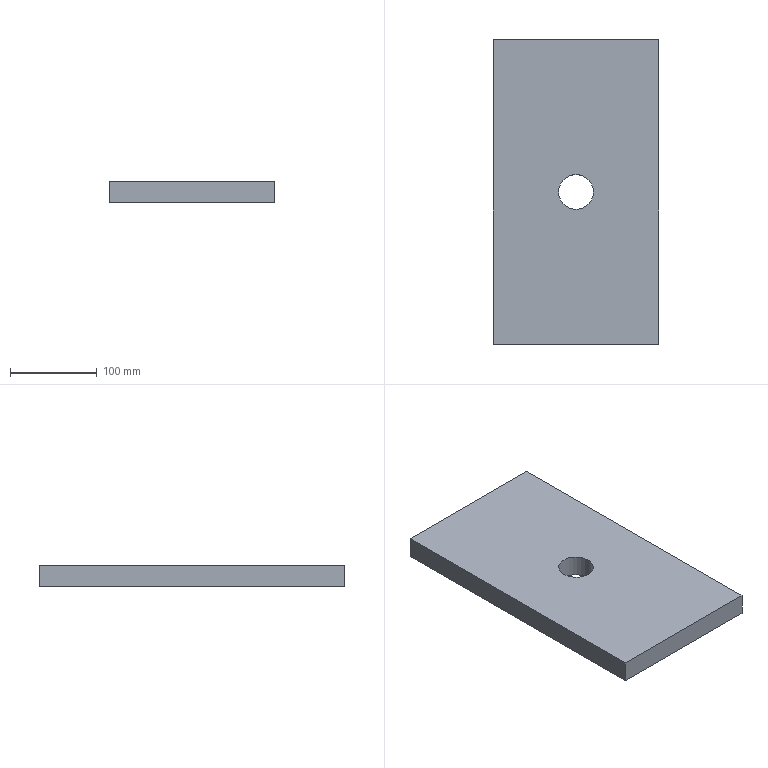Part | STEP file | Sprocket mounting plate XG | 1 solid | 8 faces | box 190 x 350 x 25 mm | volume 1631084 mm3 | plane 6 | cylinder 2 | commonest cylinder face diameters 40 x2
STEP:
#1=CARTESIAN_POINT('',(0.,0.,0.));
#2=DIRECTION('',(0.,0.,1.));
#3=DIRECTION('',(1.,0.,0.));
#4=AXIS2_PLACEMENT_3D('',#1,#2,#3);
#5=CARTESIAN_POINT('',(20.,0.,0.));
#6=VERTEX_POINT('',#5);
#7=CARTESIAN_POINT('',(20.,0.,25.));
#8=VERTEX_POINT('',#7);
#9=CARTESIAN_POINT('',(20.,0.,0.));
#10=DIRECTION('',(0.,0.,1.));
#11=VECTOR('',#10,1.);
#12=LINE('',#9,#11);
#13=CARTESIAN_POINT('',(0.,0.,0.));
#14=DIRECTION('',(0.,0.,1.));
#15=DIRECTION('',(1.,0.,0.));
#16=AXIS2_PLACEMENT_3D('',#13,#14,#15);
#17=CYLINDRICAL_SURFACE('',#16,20.);
#18=CARTESIAN_POINT('',(6.283,0.));
#19=DIRECTION('',(0.,1.));
#20=VECTOR('',#19,1.);
#21=LINE('',#18,#20);
#22=(GEOMETRIC_REPRESENTATION_CONTEXT(2)PARAMETRIC_REPRESENTATION_CONTEXT()REPRESENTATION_CONTEXT('',''));
#23=DEFINITIONAL_REPRESENTATION('',(#21),#22);
#24=PCURVE('',#17,#23);
#25=CARTESIAN_POINT('',(0.,0.,0.));
#26=DIRECTION('',(0.,0.,1.));
#27=DIRECTION('',(1.,0.,0.));
#28=AXIS2_PLACEMENT_3D('',#25,#26,#27);
#29=CYLINDRICAL_SURFACE('',#28,20.);
#30=CARTESIAN_POINT('',(0.,0.));
#31=DIRECTION('',(0.,1.));
#32=VECTOR('',#31,1.);
#33=LINE('',#30,#32);
#34=(GEOMETRIC_REPRESENTATION_CONTEXT(2)PARAMETRIC_REPRESENTATION_CONTEXT()REPRESENTATION_CONTEXT('',''));
#35=DEFINITIONAL_REPRESENTATION('',(#33),#34);
#36=PCURVE('',#29,#35);
#37=SURFACE_CURVE('',#12,(#24,#36),.PCURVE_S1.);
#38=EDGE_CURVE('',#6,#8,#37,.T.);
#39=ORIENTED_EDGE('',*,*,#38,.T.);
#40=CARTESIAN_POINT('',(-20.,0.,25.));
#41=VERTEX_POINT('',#40);
#42=CARTESIAN_POINT('',(0.,0.,25.));
#43=DIRECTION('',(0.,0.,1.));
#44=DIRECTION('',(1.,0.,0.));
#45=AXIS2_PLACEMENT_3D('',#42,#43,#44);
#46=CIRCLE('',#45,20.);
#47=CARTESIAN_POINT('',(0.,25.));
#48=DIRECTION('',(1.,0.));
#49=VECTOR('',#48,1.);
#50=LINE('',#47,#49);
#51=(GEOMETRIC_REPRESENTATION_CONTEXT(2)PARAMETRIC_REPRESENTATION_CONTEXT()REPRESENTATION_CONTEXT('',''));
#52=DEFINITIONAL_REPRESENTATION('',(#50),#51);
#53=PCURVE('',#17,#52);
#54=CARTESIAN_POINT('',(0.,0.,25.));
#55=DIRECTION('',(0.,0.,1.));
#56=DIRECTION('',(1.,0.,0.));
#57=AXIS2_PLACEMENT_3D('',#54,#55,#56);
#58=PLANE('',#57);
#59=CARTESIAN_POINT('',(0.,0.));
#60=DIRECTION('',(1.,0.));
#61=AXIS2_PLACEMENT_2D('',#59,#60);
#62=CIRCLE('',#61,20.);
#63=(GEOMETRIC_REPRESENTATION_CONTEXT(2)PARAMETRIC_REPRESENTATION_CONTEXT()REPRESENTATION_CONTEXT('',''));
#64=DEFINITIONAL_REPRESENTATION('',(#62),#63);
#65=PCURVE('',#58,#64);
#66=SURFACE_CURVE('',#46,(#53,#65),.PCURVE_S1.);
#67=EDGE_CURVE('',#41,#8,#66,.T.);
#68=ORIENTED_EDGE('',*,*,#67,.F.);
#69=CARTESIAN_POINT('',(-20.,0.,0.));
#70=VERTEX_POINT('',#69);
#71=CARTESIAN_POINT('',(-20.,0.,0.));
#72=DIRECTION('',(0.,0.,1.));
#73=VECTOR('',#72,1.);
#74=LINE('',#71,#73);
#75=CARTESIAN_POINT('',(3.142,0.));
#76=DIRECTION('',(0.,1.));
#77=VECTOR('',#76,1.);
#78=LINE('',#75,#77);
#79=(GEOMETRIC_REPRESENTATION_CONTEXT(2)PARAMETRIC_REPRESENTATION_CONTEXT()REPRESENTATION_CONTEXT('',''));
#80=DEFINITIONAL_REPRESENTATION('',(#78),#79);
#81=PCURVE('',#17,#80);
#82=CARTESIAN_POINT('',(3.142,0.));
#83=DIRECTION('',(0.,1.));
#84=VECTOR('',#83,1.);
#85=LINE('',#82,#84);
#86=(GEOMETRIC_REPRESENTATION_CONTEXT(2)PARAMETRIC_REPRESENTATION_CONTEXT()REPRESENTATION_CONTEXT('',''));
#87=DEFINITIONAL_REPRESENTATION('',(#85),#86);
#88=PCURVE('',#29,#87);
#89=SURFACE_CURVE('',#74,(#81,#88),.PCURVE_S1.);
#90=EDGE_CURVE('',#70,#41,#89,.T.);
#91=ORIENTED_EDGE('',*,*,#90,.F.);
#92=CARTESIAN_POINT('',(0.,0.,0.));
#93=DIRECTION('',(0.,0.,1.));
#94=DIRECTION('',(1.,0.,0.));
#95=AXIS2_PLACEMENT_3D('',#92,#93,#94);
#96=CIRCLE('',#95,20.);
#97=CARTESIAN_POINT('',(0.,0.));
#98=DIRECTION('',(1.,0.));
#99=VECTOR('',#98,1.);
#100=LINE('',#97,#99);
#101=(GEOMETRIC_REPRESENTATION_CONTEXT(2)PARAMETRIC_REPRESENTATION_CONTEXT()REPRESENTATION_CONTEXT('',''));
#102=DEFINITIONAL_REPRESENTATION('',(#100),#101);
#103=PCURVE('',#17,#102);
#104=CARTESIAN_POINT('',(0.,0.,0.));
#105=DIRECTION('',(0.,0.,1.));
#106=DIRECTION('',(1.,0.,0.));
#107=AXIS2_PLACEMENT_3D('',#104,#105,#106);
#108=PLANE('',#107);
#109=CARTESIAN_POINT('',(0.,0.));
#110=DIRECTION('',(1.,0.));
#111=AXIS2_PLACEMENT_2D('',#109,#110);
#112=CIRCLE('',#111,20.);
#113=(GEOMETRIC_REPRESENTATION_CONTEXT(2)PARAMETRIC_REPRESENTATION_CONTEXT()REPRESENTATION_CONTEXT('',''));
#114=DEFINITIONAL_REPRESENTATION('',(#112),#113);
#115=PCURVE('',#108,#114);
#116=SURFACE_CURVE('',#96,(#103,#115),.PCURVE_S1.);
#117=EDGE_CURVE('',#70,#6,#116,.T.);
#118=ORIENTED_EDGE('',*,*,#117,.T.);
#119=EDGE_LOOP('',(#39,#68,#91,#118));
#120=FACE_BOUND('',#119,.F.);
#121=ADVANCED_FACE('',(#120),#17,.F.);
#122=CARTESIAN_POINT('',(-95.,175.,0.));
#123=VERTEX_POINT('',#122);
#124=CARTESIAN_POINT('',(-95.,-175.,0.));
#125=VERTEX_POINT('',#124);
#126=CARTESIAN_POINT('',(-95.,175.,0.));
#127=DIRECTION('',(0.,-1.,0.));
#128=VECTOR('',#127,1.);
#129=LINE('',#126,#128);
#130=CARTESIAN_POINT('',(-95.,175.,25.));
#131=DIRECTION('',(1.,0.,0.));
#132=DIRECTION('',(0.,0.,-1.));
#133=AXIS2_PLACEMENT_3D('',#130,#131,#132);
#134=PLANE('',#133);
#135=CARTESIAN_POINT('',(25.,0.));
#136=DIRECTION('',(0.,-1.));
#137=VECTOR('',#136,1.);
#138=LINE('',#135,#137);
#139=(GEOMETRIC_REPRESENTATION_CONTEXT(2)PARAMETRIC_REPRESENTATION_CONTEXT()REPRESENTATION_CONTEXT('',''));
#140=DEFINITIONAL_REPRESENTATION('',(#138),#139);
#141=PCURVE('',#134,#140);
#142=CARTESIAN_POINT('',(-95.,175.));
#143=DIRECTION('',(0.,-1.));
#144=VECTOR('',#143,1.);
#145=LINE('',#142,#144);
#146=(GEOMETRIC_REPRESENTATION_CONTEXT(2)PARAMETRIC_REPRESENTATION_CONTEXT()REPRESENTATION_CONTEXT('',''));
#147=DEFINITIONAL_REPRESENTATION('',(#145),#146);
#148=PCURVE('',#108,#147);
#149=SURFACE_CURVE('',#129,(#141,#148),.PCURVE_S1.);
#150=EDGE_CURVE('',#123,#125,#149,.T.);
#151=ORIENTED_EDGE('',*,*,#150,.T.);
#152=CARTESIAN_POINT('',(-95.,-175.,25.));
#153=VERTEX_POINT('',#152);
#154=CARTESIAN_POINT('',(-95.,-175.,25.));
#155=DIRECTION('',(0.,0.,-1.));
#156=VECTOR('',#155,1.);
#157=LINE('',#154,#156);
#158=CARTESIAN_POINT('',(0.,-350.));
#159=DIRECTION('',(1.,0.));
#160=VECTOR('',#159,1.);
#161=LINE('',#158,#160);
#162=(GEOMETRIC_REPRESENTATION_CONTEXT(2)PARAMETRIC_REPRESENTATION_CONTEXT()REPRESENTATION_CONTEXT('',''));
#163=DEFINITIONAL_REPRESENTATION('',(#161),#162);
#164=PCURVE('',#134,#163);
#165=CARTESIAN_POINT('',(-95.,-175.,25.));
#166=DIRECTION('',(0.,1.,0.));
#167=DIRECTION('',(0.,0.,1.));
#168=AXIS2_PLACEMENT_3D('',#165,#166,#167);
#169=PLANE('',#168);
#170=CARTESIAN_POINT('',(0.,0.));
#171=DIRECTION('',(-1.,0.));
#172=VECTOR('',#171,1.);
#173=LINE('',#170,#172);
#174=(GEOMETRIC_REPRESENTATION_CONTEXT(2)PARAMETRIC_REPRESENTATION_CONTEXT()REPRESENTATION_CONTEXT('',''));
#175=DEFINITIONAL_REPRESENTATION('',(#173),#174);
#176=PCURVE('',#169,#175);
#177=SURFACE_CURVE('',#157,(#164,#176),.PCURVE_S1.);
#178=EDGE_CURVE('',#153,#125,#177,.T.);
#179=ORIENTED_EDGE('',*,*,#178,.F.);
#180=CARTESIAN_POINT('',(-95.,175.,25.));
#181=VERTEX_POINT('',#180);
#182=CARTESIAN_POINT('',(-95.,175.,25.));
#183=DIRECTION('',(0.,-1.,0.));
#184=VECTOR('',#183,1.);
#185=LINE('',#182,#184);
#186=CARTESIAN_POINT('',(0.,0.));
#187=DIRECTION('',(0.,-1.));
#188=VECTOR('',#187,1.);
#189=LINE('',#186,#188);
#190=(GEOMETRIC_REPRESENTATION_CONTEXT(2)PARAMETRIC_REPRESENTATION_CONTEXT()REPRESENTATION_CONTEXT('',''));
#191=DEFINITIONAL_REPRESENTATION('',(#189),#190);
#192=PCURVE('',#134,#191);
#193=CARTESIAN_POINT('',(-95.,175.));
#194=DIRECTION('',(0.,-1.));
#195=VECTOR('',#194,1.);
#196=LINE('',#193,#195);
#197=(GEOMETRIC_REPRESENTATION_CONTEXT(2)PARAMETRIC_REPRESENTATION_CONTEXT()REPRESENTATION_CONTEXT('',''));
#198=DEFINITIONAL_REPRESENTATION('',(#196),#197);
#199=PCURVE('',#58,#198);
#200=SURFACE_CURVE('',#185,(#192,#199),.PCURVE_S1.);
#201=EDGE_CURVE('',#181,#153,#200,.T.);
#202=ORIENTED_EDGE('',*,*,#201,.F.);
#203=CARTESIAN_POINT('',(-95.,175.,25.));
#204=DIRECTION('',(0.,0.,-1.));
#205=VECTOR('',#204,1.);
#206=LINE('',#203,#205);
#207=CARTESIAN_POINT('',(0.,0.));
#208=DIRECTION('',(1.,0.));
#209=VECTOR('',#208,1.);
#210=LINE('',#207,#209);
#211=(GEOMETRIC_REPRESENTATION_CONTEXT(2)PARAMETRIC_REPRESENTATION_CONTEXT()REPRESENTATION_CONTEXT('',''));
#212=DEFINITIONAL_REPRESENTATION('',(#210),#211);
#213=PCURVE('',#134,#212);
#214=CARTESIAN_POINT('',(-95.,175.,25.));
#215=DIRECTION('',(0.,-1.,0.));
#216=DIRECTION('',(0.,0.,-1.));
#217=AXIS2_PLACEMENT_3D('',#214,#215,#216);
#218=PLANE('',#217);
#219=CARTESIAN_POINT('',(0.,0.));
#220=DIRECTION('',(1.,0.));
#221=VECTOR('',#220,1.);
#222=LINE('',#219,#221);
#223=(GEOMETRIC_REPRESENTATION_CONTEXT(2)PARAMETRIC_REPRESENTATION_CONTEXT()REPRESENTATION_CONTEXT('',''));
#224=DEFINITIONAL_REPRESENTATION('',(#222),#223);
#225=PCURVE('',#218,#224);
#226=SURFACE_CURVE('',#206,(#213,#225),.PCURVE_S1.);
#227=EDGE_CURVE('',#181,#123,#226,.T.);
#228=ORIENTED_EDGE('',*,*,#227,.T.);
#229=EDGE_LOOP('',(#151,#179,#202,#228));
#230=FACE_BOUND('',#229,.T.);
#231=ADVANCED_FACE('',(#230),#134,.F.);
#232=CARTESIAN_POINT('',(95.,-175.,0.));
#233=VERTEX_POINT('',#232);
#234=CARTESIAN_POINT('',(-95.,-175.,0.));
#235=DIRECTION('',(1.,0.,0.));
#236=VECTOR('',#235,1.);
#237=LINE('',#234,#236);
#238=CARTESIAN_POINT('',(-25.,0.));
#239=DIRECTION('',(0.,1.));
#240=VECTOR('',#239,1.);
#241=LINE('',#238,#240);
#242=(GEOMETRIC_REPRESENTATION_CONTEXT(2)PARAMETRIC_REPRESENTATION_CONTEXT()REPRESENTATION_CONTEXT('',''));
#243=DEFINITIONAL_REPRESENTATION('',(#241),#242);
#244=PCURVE('',#169,#243);
#245=CARTESIAN_POINT('',(-95.,-175.));
#246=DIRECTION('',(1.,0.));
#247=VECTOR('',#246,1.);
#248=LINE('',#245,#247);
#249=(GEOMETRIC_REPRESENTATION_CONTEXT(2)PARAMETRIC_REPRESENTATION_CONTEXT()REPRESENTATION_CONTEXT('',''));
#250=DEFINITIONAL_REPRESENTATION('',(#248),#249);
#251=PCURVE('',#108,#250);
#252=SURFACE_CURVE('',#237,(#244,#251),.PCURVE_S1.);
#253=EDGE_CURVE('',#125,#233,#252,.T.);
#254=ORIENTED_EDGE('',*,*,#253,.T.);
#255=CARTESIAN_POINT('',(95.,-175.,25.));
#256=VERTEX_POINT('',#255);
#257=CARTESIAN_POINT('',(95.,-175.,25.));
#258=DIRECTION('',(0.,0.,-1.));
#259=VECTOR('',#258,1.);
#260=LINE('',#257,#259);
#261=CARTESIAN_POINT('',(0.,190.));
#262=DIRECTION('',(-1.,0.));
#263=VECTOR('',#262,1.);
#264=LINE('',#261,#263);
#265=(GEOMETRIC_REPRESENTATION_CONTEXT(2)PARAMETRIC_REPRESENTATION_CONTEXT()REPRESENTATION_CONTEXT('',''));
#266=DEFINITIONAL_REPRESENTATION('',(#264),#265);
#267=PCURVE('',#169,#266);
#268=CARTESIAN_POINT('',(95.,175.,25.));
#269=DIRECTION('',(-1.,0.,0.));
#270=DIRECTION('',(0.,0.,1.));
#271=AXIS2_PLACEMENT_3D('',#268,#269,#270);
#272=PLANE('',#271);
#273=CARTESIAN_POINT('',(0.,-350.));
#274=DIRECTION('',(-1.,0.));
#275=VECTOR('',#274,1.);
#276=LINE('',#273,#275);
#277=(GEOMETRIC_REPRESENTATION_CONTEXT(2)PARAMETRIC_REPRESENTATION_CONTEXT()REPRESENTATION_CONTEXT('',''));
#278=DEFINITIONAL_REPRESENTATION('',(#276),#277);
#279=PCURVE('',#272,#278);
#280=SURFACE_CURVE('',#260,(#267,#279),.PCURVE_S1.);
#281=EDGE_CURVE('',#256,#233,#280,.T.);
#282=ORIENTED_EDGE('',*,*,#281,.F.);
#283=CARTESIAN_POINT('',(-95.,-175.,25.));
#284=DIRECTION('',(1.,0.,0.));
#285=VECTOR('',#284,1.);
#286=LINE('',#283,#285);
#287=CARTESIAN_POINT('',(0.,0.));
#288=DIRECTION('',(0.,1.));
#289=VECTOR('',#288,1.);
#290=LINE('',#287,#289);
#291=(GEOMETRIC_REPRESENTATION_CONTEXT(2)PARAMETRIC_REPRESENTATION_CONTEXT()REPRESENTATION_CONTEXT('',''));
#292=DEFINITIONAL_REPRESENTATION('',(#290),#291);
#293=PCURVE('',#169,#292);
#294=CARTESIAN_POINT('',(-95.,-175.));
#295=DIRECTION('',(1.,0.));
#296=VECTOR('',#295,1.);
#297=LINE('',#294,#296);
#298=(GEOMETRIC_REPRESENTATION_CONTEXT(2)PARAMETRIC_REPRESENTATION_CONTEXT()REPRESENTATION_CONTEXT('',''));
#299=DEFINITIONAL_REPRESENTATION('',(#297),#298);
#300=PCURVE('',#58,#299);
#301=SURFACE_CURVE('',#286,(#293,#300),.PCURVE_S1.);
#302=EDGE_CURVE('',#153,#256,#301,.T.);
#303=ORIENTED_EDGE('',*,*,#302,.F.);
#304=ORIENTED_EDGE('',*,*,#178,.T.);
#305=EDGE_LOOP('',(#254,#282,#303,#304));
#306=FACE_BOUND('',#305,.T.);
#307=ADVANCED_FACE('',(#306),#169,.F.);
#308=CARTESIAN_POINT('',(95.,175.,0.));
#309=VERTEX_POINT('',#308);
#310=CARTESIAN_POINT('',(95.,175.,0.));
#311=DIRECTION('',(0.,1.,0.));
#312=VECTOR('',#311,1.);
#313=LINE('',#310,#312);
#314=CARTESIAN_POINT('',(-25.,0.));
#315=DIRECTION('',(0.,1.));
#316=VECTOR('',#315,1.);
#317=LINE('',#314,#316);
#318=(GEOMETRIC_REPRESENTATION_CONTEXT(2)PARAMETRIC_REPRESENTATION_CONTEXT()REPRESENTATION_CONTEXT('',''));
#319=DEFINITIONAL_REPRESENTATION('',(#317),#318);
#320=PCURVE('',#272,#319);
#321=CARTESIAN_POINT('',(95.,175.));
#322=DIRECTION('',(0.,1.));
#323=VECTOR('',#322,1.);
#324=LINE('',#321,#323);
#325=(GEOMETRIC_REPRESENTATION_CONTEXT(2)PARAMETRIC_REPRESENTATION_CONTEXT()REPRESENTATION_CONTEXT('',''));
#326=DEFINITIONAL_REPRESENTATION('',(#324),#325);
#327=PCURVE('',#108,#326);
#328=SURFACE_CURVE('',#313,(#320,#327),.PCURVE_S1.);
#329=EDGE_CURVE('',#233,#309,#328,.T.);
#330=ORIENTED_EDGE('',*,*,#329,.T.);
#331=CARTESIAN_POINT('',(95.,175.,25.));
#332=VERTEX_POINT('',#331);
#333=CARTESIAN_POINT('',(95.,175.,25.));
#334=DIRECTION('',(0.,0.,-1.));
#335=VECTOR('',#334,1.);
#336=LINE('',#333,#335);
#337=CARTESIAN_POINT('',(0.,0.));
#338=DIRECTION('',(-1.,0.));
#339=VECTOR('',#338,1.);
#340=LINE('',#337,#339);
#341=(GEOMETRIC_REPRESENTATION_CONTEXT(2)PARAMETRIC_REPRESENTATION_CONTEXT()REPRESENTATION_CONTEXT('',''));
#342=DEFINITIONAL_REPRESENTATION('',(#340),#341);
#343=PCURVE('',#272,#342);
#344=CARTESIAN_POINT('',(0.,190.));
#345=DIRECTION('',(1.,0.));
#346=VECTOR('',#345,1.);
#347=LINE('',#344,#346);
#348=(GEOMETRIC_REPRESENTATION_CONTEXT(2)PARAMETRIC_REPRESENTATION_CONTEXT()REPRESENTATION_CONTEXT('',''));
#349=DEFINITIONAL_REPRESENTATION('',(#347),#348);
#350=PCURVE('',#218,#349);
#351=SURFACE_CURVE('',#336,(#343,#350),.PCURVE_S1.);
#352=EDGE_CURVE('',#332,#309,#351,.T.);
#353=ORIENTED_EDGE('',*,*,#352,.F.);
#354=CARTESIAN_POINT('',(95.,175.,25.));
#355=DIRECTION('',(0.,1.,0.));
#356=VECTOR('',#355,1.);
#357=LINE('',#354,#356);
#358=CARTESIAN_POINT('',(0.,0.));
#359=DIRECTION('',(0.,1.));
#360=VECTOR('',#359,1.);
#361=LINE('',#358,#360);
#362=(GEOMETRIC_REPRESENTATION_CONTEXT(2)PARAMETRIC_REPRESENTATION_CONTEXT()REPRESENTATION_CONTEXT('',''));
#363=DEFINITIONAL_REPRESENTATION('',(#361),#362);
#364=PCURVE('',#272,#363);
#365=CARTESIAN_POINT('',(95.,175.));
#366=DIRECTION('',(0.,1.));
#367=VECTOR('',#366,1.);
#368=LINE('',#365,#367);
#369=(GEOMETRIC_REPRESENTATION_CONTEXT(2)PARAMETRIC_REPRESENTATION_CONTEXT()REPRESENTATION_CONTEXT('',''));
#370=DEFINITIONAL_REPRESENTATION('',(#368),#369);
#371=PCURVE('',#58,#370);
#372=SURFACE_CURVE('',#357,(#364,#371),.PCURVE_S1.);
#373=EDGE_CURVE('',#256,#332,#372,.T.);
#374=ORIENTED_EDGE('',*,*,#373,.F.);
#375=ORIENTED_EDGE('',*,*,#281,.T.);
#376=EDGE_LOOP('',(#330,#353,#374,#375));
#377=FACE_BOUND('',#376,.T.);
#378=ADVANCED_FACE('',(#377),#272,.F.);
#379=CARTESIAN_POINT('',(-95.,175.,0.));
#380=DIRECTION('',(-1.,0.,0.));
#381=VECTOR('',#380,1.);
#382=LINE('',#379,#381);
#383=CARTESIAN_POINT('',(25.,0.));
#384=DIRECTION('',(0.,-1.));
#385=VECTOR('',#384,1.);
#386=LINE('',#383,#385);
#387=(GEOMETRIC_REPRESENTATION_CONTEXT(2)PARAMETRIC_REPRESENTATION_CONTEXT()REPRESENTATION_CONTEXT('',''));
#388=DEFINITIONAL_REPRESENTATION('',(#386),#387);
#389=PCURVE('',#218,#388);
#390=CARTESIAN_POINT('',(-95.,175.));
#391=DIRECTION('',(-1.,0.));
#392=VECTOR('',#391,1.);
#393=LINE('',#390,#392);
#394=(GEOMETRIC_REPRESENTATION_CONTEXT(2)PARAMETRIC_REPRESENTATION_CONTEXT()REPRESENTATION_CONTEXT('',''));
#395=DEFINITIONAL_REPRESENTATION('',(#393),#394);
#396=PCURVE('',#108,#395);
#397=SURFACE_CURVE('',#382,(#389,#396),.PCURVE_S1.);
#398=EDGE_CURVE('',#309,#123,#397,.T.);
#399=ORIENTED_EDGE('',*,*,#398,.T.);
#400=ORIENTED_EDGE('',*,*,#227,.F.);
#401=CARTESIAN_POINT('',(-95.,175.,25.));
#402=DIRECTION('',(-1.,0.,0.));
#403=VECTOR('',#402,1.);
#404=LINE('',#401,#403);
#405=CARTESIAN_POINT('',(0.,0.));
#406=DIRECTION('',(0.,-1.));
#407=VECTOR('',#406,1.);
#408=LINE('',#405,#407);
#409=(GEOMETRIC_REPRESENTATION_CONTEXT(2)PARAMETRIC_REPRESENTATION_CONTEXT()REPRESENTATION_CONTEXT('',''));
#410=DEFINITIONAL_REPRESENTATION('',(#408),#409);
#411=PCURVE('',#218,#410);
#412=CARTESIAN_POINT('',(-95.,175.));
#413=DIRECTION('',(-1.,0.));
#414=VECTOR('',#413,1.);
#415=LINE('',#412,#414);
#416=(GEOMETRIC_REPRESENTATION_CONTEXT(2)PARAMETRIC_REPRESENTATION_CONTEXT()REPRESENTATION_CONTEXT('',''));
#417=DEFINITIONAL_REPRESENTATION('',(#415),#416);
#418=PCURVE('',#58,#417);
#419=SURFACE_CURVE('',#404,(#411,#418),.PCURVE_S1.);
#420=EDGE_CURVE('',#332,#181,#419,.T.);
#421=ORIENTED_EDGE('',*,*,#420,.F.);
#422=ORIENTED_EDGE('',*,*,#352,.T.);
#423=EDGE_LOOP('',(#399,#400,#421,#422));
#424=FACE_BOUND('',#423,.T.);
#425=ADVANCED_FACE('',(#424),#218,.F.);
#426=CARTESIAN_POINT('',(0.,0.,25.));
#427=DIRECTION('',(0.,0.,1.));
#428=DIRECTION('',(1.,0.,0.));
#429=AXIS2_PLACEMENT_3D('',#426,#427,#428);
#430=CIRCLE('',#429,20.);
#431=CARTESIAN_POINT('',(0.,0.));
#432=DIRECTION('',(1.,0.));
#433=AXIS2_PLACEMENT_2D('',#431,#432);
#434=CIRCLE('',#433,20.);
#435=(GEOMETRIC_REPRESENTATION_CONTEXT(2)PARAMETRIC_REPRESENTATION_CONTEXT()REPRESENTATION_CONTEXT('',''));
#436=DEFINITIONAL_REPRESENTATION('',(#434),#435);
#437=PCURVE('',#58,#436);
#438=CARTESIAN_POINT('',(0.,25.));
#439=DIRECTION('',(1.,0.));
#440=VECTOR('',#439,1.);
#441=LINE('',#438,#440);
#442=(GEOMETRIC_REPRESENTATION_CONTEXT(2)PARAMETRIC_REPRESENTATION_CONTEXT()REPRESENTATION_CONTEXT('',''));
#443=DEFINITIONAL_REPRESENTATION('',(#441),#442);
#444=PCURVE('',#29,#443);
#445=SURFACE_CURVE('',#430,(#437,#444),.PCURVE_S1.);
#446=EDGE_CURVE('',#8,#41,#445,.T.);
#447=ORIENTED_EDGE('',*,*,#446,.F.);
#448=ORIENTED_EDGE('',*,*,#67,.F.);
#449=EDGE_LOOP('',(#447,#448));
#450=FACE_BOUND('',#449,.T.);
#451=ORIENTED_EDGE('',*,*,#201,.T.);
#452=ORIENTED_EDGE('',*,*,#302,.T.);
#453=ORIENTED_EDGE('',*,*,#373,.T.);
#454=ORIENTED_EDGE('',*,*,#420,.T.);
#455=EDGE_LOOP('',(#451,#452,#453,#454));
#456=FACE_BOUND('',#455,.T.);
#457=ADVANCED_FACE('',(#450,#456),#58,.T.);
#458=CARTESIAN_POINT('',(0.,0.,0.));
#459=DIRECTION('',(0.,0.,1.));
#460=DIRECTION('',(1.,0.,0.));
#461=AXIS2_PLACEMENT_3D('',#458,#459,#460);
#462=CIRCLE('',#461,20.);
#463=CARTESIAN_POINT('',(0.,0.));
#464=DIRECTION('',(1.,0.));
#465=AXIS2_PLACEMENT_2D('',#463,#464);
#466=CIRCLE('',#465,20.);
#467=(GEOMETRIC_REPRESENTATION_CONTEXT(2)PARAMETRIC_REPRESENTATION_CONTEXT()REPRESENTATION_CONTEXT('',''));
#468=DEFINITIONAL_REPRESENTATION('',(#466),#467);
#469=PCURVE('',#108,#468);
#470=CARTESIAN_POINT('',(0.,0.));
#471=DIRECTION('',(1.,0.));
#472=VECTOR('',#471,1.);
#473=LINE('',#470,#472);
#474=(GEOMETRIC_REPRESENTATION_CONTEXT(2)PARAMETRIC_REPRESENTATION_CONTEXT()REPRESENTATION_CONTEXT('',''));
#475=DEFINITIONAL_REPRESENTATION('',(#473),#474);
#476=PCURVE('',#29,#475);
#477=SURFACE_CURVE('',#462,(#469,#476),.PCURVE_S1.);
#478=EDGE_CURVE('',#6,#70,#477,.T.);
#479=ORIENTED_EDGE('',*,*,#478,.T.);
#480=ORIENTED_EDGE('',*,*,#117,.T.);
#481=EDGE_LOOP('',(#479,#480));
#482=FACE_BOUND('',#481,.T.);
#483=ORIENTED_EDGE('',*,*,#150,.F.);
#484=ORIENTED_EDGE('',*,*,#398,.F.);
#485=ORIENTED_EDGE('',*,*,#329,.F.);
#486=ORIENTED_EDGE('',*,*,#253,.F.);
#487=EDGE_LOOP('',(#483,#484,#485,#486));
#488=FACE_BOUND('',#487,.T.);
#489=ADVANCED_FACE('',(#482,#488),#108,.F.);
#490=ORIENTED_EDGE('',*,*,#446,.F.);
#491=ORIENTED_EDGE('',*,*,#38,.F.);
#492=ORIENTED_EDGE('',*,*,#478,.T.);
#493=ORIENTED_EDGE('',*,*,#90,.T.);
#494=EDGE_LOOP('',(#490,#491,#492,#493));
#495=FACE_BOUND('',#494,.F.);
#496=ADVANCED_FACE('',(#495),#29,.F.);
#497=CLOSED_SHELL('',(#121,#231,#307,#378,#425,#457,#489,#496));
#498=MANIFOLD_SOLID_BREP('',#497);
#499=(LENGTH_UNIT()NAMED_UNIT(*)SI_UNIT(.MILLI.,.METRE.));
#500=UNCERTAINTY_MEASURE_WITH_UNIT(LENGTH_MEASURE(0.0000001),#499,'','');
#501=(NAMED_UNIT(*)PLANE_ANGLE_UNIT()SI_UNIT($,.RADIAN.));
#502=(NAMED_UNIT(*)SI_UNIT($,.STERADIAN.)SOLID_ANGLE_UNIT());
#503=(GEOMETRIC_REPRESENTATION_CONTEXT(3)GLOBAL_UNCERTAINTY_ASSIGNED_CONTEXT((#500))GLOBAL_UNIT_ASSIGNED_CONTEXT((#499,#501,#502))REPRESENTATION_CONTEXT('',''));
#504=ADVANCED_BREP_SHAPE_REPRESENTATION('',(#4,#498),#503);